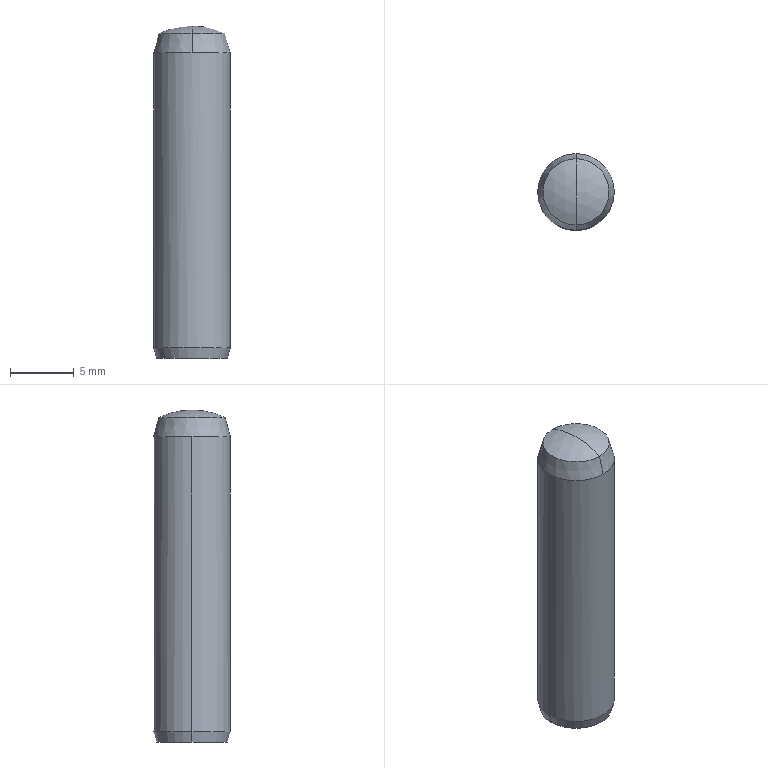Part | SolidWorks | features Chamfer 2, Cut 2, Extrusion 1, RevCut 1, Revolution 1 | 1 solid | 17 faces | box 6 x 6 x 26 mm | volume 614.212 mm3 | cone 8 | cylinder 6 | sphere 2 | plane 1 | commonest cylinder face diameters 3.464 x2 4.3 x2 6 x2
STEP:
#1=CARTESIAN_POINT('',(1.732,0.,1.418));
#2=VERTEX_POINT('',#1);
#3=CARTESIAN_POINT('',(-1.732,0.,1.418));
#4=VERTEX_POINT('',#3);
#5=CARTESIAN_POINT('',(0.,0.,1.418));
#6=DIRECTION('',(0.,0.,-1.));
#7=DIRECTION('',(-1.,0.,0.));
#8=AXIS2_PLACEMENT_3D('',#5,#6,#7);
#9=CIRCLE('',#8,1.732);
#10=EDGE_CURVE('',#2,#4,#9,.T.);
#11=ORIENTED_EDGE('',*,*,#10,.F.);
#12=CARTESIAN_POINT('',(2.15,0.,1.));
#13=VERTEX_POINT('',#12);
#14=CARTESIAN_POINT('',(2.15,0.,1.));
#15=DIRECTION('',(0.7071,0.,-0.7071));
#16=VECTOR('',#15,1000.);
#17=LINE('',#14,#16);
#18=EDGE_CURVE('',#2,#13,#17,.T.);
#19=ORIENTED_EDGE('',*,*,#18,.T.);
#20=CARTESIAN_POINT('',(-2.15,0.,1.));
#21=VERTEX_POINT('',#20);
#22=CARTESIAN_POINT('',(0.,0.,1.));
#23=DIRECTION('',(0.,0.,-1.));
#24=DIRECTION('',(-1.,0.,0.));
#25=AXIS2_PLACEMENT_3D('',#22,#23,#24);
#26=CIRCLE('',#25,2.15);
#27=EDGE_CURVE('',#13,#21,#26,.T.);
#28=ORIENTED_EDGE('',*,*,#27,.T.);
#29=CARTESIAN_POINT('',(-2.15,0.,1.));
#30=DIRECTION('',(-0.7071,0.,-0.7071));
#31=VECTOR('',#30,1000.);
#32=LINE('',#29,#31);
#33=EDGE_CURVE('',#4,#21,#32,.T.);
#34=ORIENTED_EDGE('',*,*,#33,.F.);
#35=EDGE_LOOP('',(#11,#19,#28,#34));
#36=FACE_OUTER_BOUND('',#35,.T.);
#37=CARTESIAN_POINT('',(0.,0.,1.));
#38=DIRECTION('',(0.,0.,-1.));
#39=DIRECTION('',(-1.,0.,0.));
#40=AXIS2_PLACEMENT_3D('',#37,#38,#39);
#41=CONICAL_SURFACE('',#40,2.15,0.7854);
#42=ADVANCED_FACE('',(#36),#41,.F.);
#43=CARTESIAN_POINT('',(-1.732,0.,10.));
#44=VERTEX_POINT('',#43);
#45=CARTESIAN_POINT('',(1.732,0.,10.));
#46=VERTEX_POINT('',#45);
#47=CARTESIAN_POINT('',(0.,0.,10.));
#48=DIRECTION('',(0.,0.,1.));
#49=DIRECTION('',(1.,0.,0.));
#50=AXIS2_PLACEMENT_3D('',#47,#48,#49);
#51=CIRCLE('',#50,1.732);
#52=EDGE_CURVE('',#44,#46,#51,.T.);
#53=ORIENTED_EDGE('',*,*,#52,.T.);
#54=CARTESIAN_POINT('',(1.732,0.,10.));
#55=DIRECTION('',(0.,0.,-1.));
#56=VECTOR('',#55,1000.);
#57=LINE('',#54,#56);
#58=EDGE_CURVE('',#46,#2,#57,.T.);
#59=ORIENTED_EDGE('',*,*,#58,.T.);
#60=ORIENTED_EDGE('',*,*,#10,.T.);
#61=CARTESIAN_POINT('',(-1.732,0.,10.));
#62=DIRECTION('',(0.,0.,-1.));
#63=VECTOR('',#62,1000.);
#64=LINE('',#61,#63);
#65=EDGE_CURVE('',#44,#4,#64,.T.);
#66=ORIENTED_EDGE('',*,*,#65,.F.);
#67=EDGE_LOOP('',(#53,#59,#60,#66));
#68=FACE_OUTER_BOUND('',#67,.T.);
#69=CARTESIAN_POINT('',(0.,0.,10.));
#70=DIRECTION('',(0.,0.,-1.));
#71=DIRECTION('',(-1.,0.,0.));
#72=AXIS2_PLACEMENT_3D('',#69,#70,#71);
#73=CYLINDRICAL_SURFACE('',#72,1.732);
#74=ADVANCED_FACE('',(#68),#73,.F.);
#75=CARTESIAN_POINT('',(0.,0.,11.));
#76=VERTEX_POINT('',#75);
#77=CARTESIAN_POINT('',(-1.732,0.,10.));
#78=DIRECTION('',(-0.866,0.,-0.5));
#79=VECTOR('',#78,1000.);
#80=LINE('',#77,#79);
#81=EDGE_CURVE('',#76,#44,#80,.T.);
#82=ORIENTED_EDGE('',*,*,#81,.F.);
#83=CARTESIAN_POINT('',(1.732,0.,10.));
#84=DIRECTION('',(0.866,0.,-0.5));
#85=VECTOR('',#84,1000.);
#86=LINE('',#83,#85);
#87=EDGE_CURVE('',#76,#46,#86,.T.);
#88=ORIENTED_EDGE('',*,*,#87,.T.);
#89=ORIENTED_EDGE('',*,*,#52,.F.);
#90=EDGE_LOOP('',(#82,#88,#89));
#91=FACE_OUTER_BOUND('',#90,.T.);
#92=CARTESIAN_POINT('',(0.,0.,10.));
#93=DIRECTION('',(0.,0.,-1.));
#94=DIRECTION('',(-1.,0.,0.));
#95=AXIS2_PLACEMENT_3D('',#92,#93,#94);
#96=CONICAL_SURFACE('',#95,1.732,1.047);
#97=ADVANCED_FACE('',(#91),#96,.F.);
#98=ORIENTED_EDGE('',*,*,#27,.F.);
#99=CARTESIAN_POINT('',(2.15,0.,0.));
#100=VERTEX_POINT('',#99);
#101=CARTESIAN_POINT('',(2.15,0.,1.));
#102=DIRECTION('',(0.,0.,-1.));
#103=VECTOR('',#102,1000.);
#104=LINE('',#101,#103);
#105=EDGE_CURVE('',#13,#100,#104,.T.);
#106=ORIENTED_EDGE('',*,*,#105,.T.);
#107=CARTESIAN_POINT('',(-2.15,0.,0.));
#108=VERTEX_POINT('',#107);
#109=CARTESIAN_POINT('',(0.,0.,0.));
#110=DIRECTION('',(0.,0.,-1.));
#111=DIRECTION('',(-1.,0.,0.));
#112=AXIS2_PLACEMENT_3D('',#109,#110,#111);
#113=CIRCLE('',#112,2.15);
#114=EDGE_CURVE('',#100,#108,#113,.T.);
#115=ORIENTED_EDGE('',*,*,#114,.T.);
#116=CARTESIAN_POINT('',(-2.15,0.,1.));
#117=DIRECTION('',(0.,0.,-1.));
#118=VECTOR('',#117,1000.);
#119=LINE('',#116,#118);
#120=EDGE_CURVE('',#21,#108,#119,.T.);
#121=ORIENTED_EDGE('',*,*,#120,.F.);
#122=EDGE_LOOP('',(#98,#106,#115,#121));
#123=FACE_OUTER_BOUND('',#122,.T.);
#124=CARTESIAN_POINT('',(0.,0.,1.));
#125=DIRECTION('',(0.,0.,-1.));
#126=DIRECTION('',(-1.,0.,0.));
#127=AXIS2_PLACEMENT_3D('',#124,#125,#126);
#128=CYLINDRICAL_SURFACE('',#127,2.15);
#129=ADVANCED_FACE('',(#123),#128,.F.);
#130=CARTESIAN_POINT('',(-2.786,0.,0.));
#131=VERTEX_POINT('',#130);
#132=CARTESIAN_POINT('',(2.786,0.,0.));
#133=VERTEX_POINT('',#132);
#134=CARTESIAN_POINT('',(0.,0.,0.));
#135=DIRECTION('',(0.,0.,-1.));
#136=DIRECTION('',(1.,0.,0.));
#137=AXIS2_PLACEMENT_3D('',#134,#135,#136);
#138=CIRCLE('',#137,2.786);
#139=EDGE_CURVE('',#131,#133,#138,.T.);
#140=ORIENTED_EDGE('',*,*,#139,.F.);
#141=CARTESIAN_POINT('',(-3.,0.,0.8));
#142=VERTEX_POINT('',#141);
#143=CARTESIAN_POINT('',(-3.,0.,0.8));
#144=DIRECTION('',(-0.2588,0.,0.9659));
#145=VECTOR('',#144,1000.);
#146=LINE('',#143,#145);
#147=EDGE_CURVE('',#131,#142,#146,.T.);
#148=ORIENTED_EDGE('',*,*,#147,.T.);
#149=CARTESIAN_POINT('',(3.,0.,0.8));
#150=VERTEX_POINT('',#149);
#151=CARTESIAN_POINT('',(0.,0.,0.8));
#152=DIRECTION('',(0.,0.,1.));
#153=DIRECTION('',(1.,0.,0.));
#154=AXIS2_PLACEMENT_3D('',#151,#152,#153);
#155=CIRCLE('',#154,3.);
#156=EDGE_CURVE('',#150,#142,#155,.T.);
#157=ORIENTED_EDGE('',*,*,#156,.F.);
#158=CARTESIAN_POINT('',(3.,0.,0.8));
#159=DIRECTION('',(0.2588,0.,0.9659));
#160=VECTOR('',#159,1000.);
#161=LINE('',#158,#160);
#162=EDGE_CURVE('',#133,#150,#161,.T.);
#163=ORIENTED_EDGE('',*,*,#162,.F.);
#164=EDGE_LOOP('',(#140,#148,#157,#163));
#165=FACE_OUTER_BOUND('',#164,.T.);
#166=CARTESIAN_POINT('',(0.,0.,0.8));
#167=DIRECTION('',(0.,0.,1.));
#168=DIRECTION('',(1.,0.,0.));
#169=AXIS2_PLACEMENT_3D('',#166,#167,#168);
#170=CONICAL_SURFACE('',#169,3.,0.2618);
#171=ADVANCED_FACE('',(#165),#170,.T.);
#172=CARTESIAN_POINT('',(0.,0.,26.));
#173=VERTEX_POINT('',#172);
#174=CARTESIAN_POINT('',(0.,2.596,25.41));
#175=VERTEX_POINT('',#174);
#176=CARTESIAN_POINT('',(0.,0.,20.));
#177=DIRECTION('',(-1.,0.,0.));
#178=DIRECTION('',(0.,0.,1.));
#179=AXIS2_PLACEMENT_3D('',#176,#177,#178);
#180=CIRCLE('',#179,6.);
#181=EDGE_CURVE('',#173,#175,#180,.T.);
#182=ORIENTED_EDGE('',*,*,#181,.F.);
#183=CARTESIAN_POINT('',(0.,-2.596,25.41));
#184=VERTEX_POINT('',#183);
#185=CARTESIAN_POINT('',(0.,0.,20.));
#186=DIRECTION('',(1.,0.,0.));
#187=DIRECTION('',(0.,1.,0.));
#188=AXIS2_PLACEMENT_3D('',#185,#186,#187);
#189=CIRCLE('',#188,6.);
#190=EDGE_CURVE('',#173,#184,#189,.T.);
#191=ORIENTED_EDGE('',*,*,#190,.T.);
#192=CARTESIAN_POINT('',(0.,0.,25.41));
#193=DIRECTION('',(0.,0.,-1.));
#194=DIRECTION('',(0.,1.,0.));
#195=AXIS2_PLACEMENT_3D('',#192,#193,#194);
#196=CIRCLE('',#195,2.596);
#197=EDGE_CURVE('',#175,#184,#196,.T.);
#198=ORIENTED_EDGE('',*,*,#197,.F.);
#199=EDGE_LOOP('',(#182,#191,#198));
#200=FACE_OUTER_BOUND('',#199,.T.);
#201=CARTESIAN_POINT('',(0.,0.,20.));
#202=DIRECTION('',(1.,0.,0.));
#203=DIRECTION('',(0.,1.,0.));
#204=AXIS2_PLACEMENT_3D('',#201,#202,#203);
#205=SPHERICAL_SURFACE('',#204,6.);
#206=ADVANCED_FACE('',(#200),#205,.T.);
#207=ORIENTED_EDGE('',*,*,#197,.T.);
#208=CARTESIAN_POINT('',(0.,-3.,23.9));
#209=VERTEX_POINT('',#208);
#210=CARTESIAN_POINT('',(0.,-3.,23.9));
#211=DIRECTION('',(0.,-0.2588,-0.9659));
#212=VECTOR('',#211,1000.);
#213=LINE('',#210,#212);
#214=EDGE_CURVE('',#184,#209,#213,.T.);
#215=ORIENTED_EDGE('',*,*,#214,.T.);
#216=CARTESIAN_POINT('',(3.,0.,23.9));
#217=VERTEX_POINT('',#216);
#218=CARTESIAN_POINT('',(0.,0.,23.9));
#219=DIRECTION('',(0.,0.,1.));
#220=DIRECTION('',(1.,0.,0.));
#221=AXIS2_PLACEMENT_3D('',#218,#219,#220);
#222=CIRCLE('',#221,3.);
#223=EDGE_CURVE('',#209,#217,#222,.T.);
#224=ORIENTED_EDGE('',*,*,#223,.T.);
#225=CARTESIAN_POINT('',(0.,3.,23.9));
#226=VERTEX_POINT('',#225);
#227=CARTESIAN_POINT('',(0.,0.,23.9));
#228=DIRECTION('',(0.,0.,1.));
#229=DIRECTION('',(1.,0.,0.));
#230=AXIS2_PLACEMENT_3D('',#227,#228,#229);
#231=CIRCLE('',#230,3.);
#232=EDGE_CURVE('',#217,#226,#231,.T.);
#233=ORIENTED_EDGE('',*,*,#232,.T.);
#234=CARTESIAN_POINT('',(0.,3.,23.9));
#235=DIRECTION('',(0.,0.2588,-0.9659));
#236=VECTOR('',#235,1000.);
#237=LINE('',#234,#236);
#238=EDGE_CURVE('',#175,#226,#237,.T.);
#239=ORIENTED_EDGE('',*,*,#238,.F.);
#240=EDGE_LOOP('',(#207,#215,#224,#233,#239));
#241=FACE_OUTER_BOUND('',#240,.T.);
#242=CARTESIAN_POINT('',(0.,0.,23.9));
#243=DIRECTION('',(0.,0.,-1.));
#244=DIRECTION('',(0.,1.,0.));
#245=AXIS2_PLACEMENT_3D('',#242,#243,#244);
#246=CONICAL_SURFACE('',#245,3.,0.2618);
#247=ADVANCED_FACE('',(#241),#246,.T.);
#248=ORIENTED_EDGE('',*,*,#232,.F.);
#249=CARTESIAN_POINT('',(3.,0.,23.9));
#250=DIRECTION('',(0.,0.,-1.));
#251=VECTOR('',#250,1000.);
#252=LINE('',#249,#251);
#253=EDGE_CURVE('',#217,#150,#252,.T.);
#254=ORIENTED_EDGE('',*,*,#253,.T.);
#255=ORIENTED_EDGE('',*,*,#156,.T.);
#256=CARTESIAN_POINT('',(-3.,0.,23.9));
#257=VERTEX_POINT('',#256);
#258=CARTESIAN_POINT('',(-3.,0.,23.9));
#259=DIRECTION('',(0.,0.,-1.));
#260=VECTOR('',#259,1000.);
#261=LINE('',#258,#260);
#262=EDGE_CURVE('',#257,#142,#261,.T.);
#263=ORIENTED_EDGE('',*,*,#262,.F.);
#264=CARTESIAN_POINT('',(0.,0.,23.9));
#265=DIRECTION('',(0.,0.,1.));
#266=DIRECTION('',(1.,0.,0.));
#267=AXIS2_PLACEMENT_3D('',#264,#265,#266);
#268=CIRCLE('',#267,3.);
#269=EDGE_CURVE('',#226,#257,#268,.T.);
#270=ORIENTED_EDGE('',*,*,#269,.F.);
#271=EDGE_LOOP('',(#248,#254,#255,#263,#270));
#272=FACE_OUTER_BOUND('',#271,.T.);
#273=CARTESIAN_POINT('',(0.,0.,23.9));
#274=DIRECTION('',(0.,0.,-1.));
#275=DIRECTION('',(-1.,0.,0.));
#276=AXIS2_PLACEMENT_3D('',#273,#274,#275);
#277=CYLINDRICAL_SURFACE('',#276,3.);
#278=ADVANCED_FACE('',(#272),#277,.T.);
#279=ORIENTED_EDGE('',*,*,#253,.F.);
#280=ORIENTED_EDGE('',*,*,#223,.F.);
#281=CARTESIAN_POINT('',(0.,0.,23.9));
#282=DIRECTION('',(0.,0.,1.));
#283=DIRECTION('',(1.,0.,0.));
#284=AXIS2_PLACEMENT_3D('',#281,#282,#283);
#285=CIRCLE('',#284,3.);
#286=EDGE_CURVE('',#257,#209,#285,.T.);
#287=ORIENTED_EDGE('',*,*,#286,.F.);
#288=ORIENTED_EDGE('',*,*,#262,.T.);
#289=CARTESIAN_POINT('',(0.,0.,0.8));
#290=DIRECTION('',(0.,0.,1.));
#291=DIRECTION('',(1.,0.,0.));
#292=AXIS2_PLACEMENT_3D('',#289,#290,#291);
#293=CIRCLE('',#292,3.);
#294=EDGE_CURVE('',#142,#150,#293,.T.);
#295=ORIENTED_EDGE('',*,*,#294,.T.);
#296=EDGE_LOOP('',(#279,#280,#287,#288,#295));
#297=FACE_OUTER_BOUND('',#296,.T.);
#298=CARTESIAN_POINT('',(0.,0.,23.9));
#299=DIRECTION('',(0.,0.,-1.));
#300=DIRECTION('',(-1.,0.,0.));
#301=AXIS2_PLACEMENT_3D('',#298,#299,#300);
#302=CYLINDRICAL_SURFACE('',#301,3.);
#303=ADVANCED_FACE('',(#297),#302,.T.);
#304=CARTESIAN_POINT('',(0.,0.,0.));
#305=DIRECTION('',(0.,0.,-1.));
#306=DIRECTION('',(-1.,0.,0.));
#307=AXIS2_PLACEMENT_3D('',#304,#305,#306);
#308=CIRCLE('',#307,2.15);
#309=EDGE_CURVE('',#108,#100,#308,.T.);
#310=ORIENTED_EDGE('',*,*,#309,.F.);
#311=ORIENTED_EDGE('',*,*,#114,.F.);
#312=EDGE_LOOP('',(#310,#311));
#313=FACE_BOUND('',#312,.T.);
#314=CARTESIAN_POINT('',(0.,0.,0.));
#315=DIRECTION('',(0.,0.,-1.));
#316=DIRECTION('',(1.,0.,0.));
#317=AXIS2_PLACEMENT_3D('',#314,#315,#316);
#318=CIRCLE('',#317,2.786);
#319=EDGE_CURVE('',#133,#131,#318,.T.);
#320=ORIENTED_EDGE('',*,*,#319,.T.);
#321=ORIENTED_EDGE('',*,*,#139,.T.);
#322=EDGE_LOOP('',(#320,#321));
#323=FACE_OUTER_BOUND('',#322,.T.);
#324=CARTESIAN_POINT('',(0.,0.,0.));
#325=DIRECTION('',(0.,0.,1.));
#326=DIRECTION('',(1.,0.,0.));
#327=AXIS2_PLACEMENT_3D('',#324,#325,#326);
#328=PLANE('',#327);
#329=ADVANCED_FACE('',(#313,#323),#328,.F.);
#330=ORIENTED_EDGE('',*,*,#214,.F.);
#331=CARTESIAN_POINT('',(0.,0.,25.41));
#332=DIRECTION('',(0.,0.,-1.));
#333=DIRECTION('',(0.,1.,0.));
#334=AXIS2_PLACEMENT_3D('',#331,#332,#333);
#335=CIRCLE('',#334,2.596);
#336=EDGE_CURVE('',#184,#175,#335,.T.);
#337=ORIENTED_EDGE('',*,*,#336,.T.);
#338=ORIENTED_EDGE('',*,*,#238,.T.);
#339=ORIENTED_EDGE('',*,*,#269,.T.);
#340=ORIENTED_EDGE('',*,*,#286,.T.);
#341=EDGE_LOOP('',(#330,#337,#338,#339,#340));
#342=FACE_OUTER_BOUND('',#341,.T.);
#343=CARTESIAN_POINT('',(0.,0.,23.9));
#344=DIRECTION('',(0.,0.,-1.));
#345=DIRECTION('',(0.,1.,0.));
#346=AXIS2_PLACEMENT_3D('',#343,#344,#345);
#347=CONICAL_SURFACE('',#346,3.,0.2618);
#348=ADVANCED_FACE('',(#342),#347,.T.);
#349=ORIENTED_EDGE('',*,*,#190,.F.);
#350=ORIENTED_EDGE('',*,*,#181,.T.);
#351=ORIENTED_EDGE('',*,*,#336,.F.);
#352=EDGE_LOOP('',(#349,#350,#351));
#353=FACE_OUTER_BOUND('',#352,.T.);
#354=CARTESIAN_POINT('',(0.,0.,20.));
#355=DIRECTION('',(1.,0.,0.));
#356=DIRECTION('',(0.,1.,0.));
#357=AXIS2_PLACEMENT_3D('',#354,#355,#356);
#358=SPHERICAL_SURFACE('',#357,6.);
#359=ADVANCED_FACE('',(#353),#358,.T.);
#360=ORIENTED_EDGE('',*,*,#147,.F.);
#361=ORIENTED_EDGE('',*,*,#319,.F.);
#362=ORIENTED_EDGE('',*,*,#162,.T.);
#363=ORIENTED_EDGE('',*,*,#294,.F.);
#364=EDGE_LOOP('',(#360,#361,#362,#363));
#365=FACE_OUTER_BOUND('',#364,.T.);
#366=CARTESIAN_POINT('',(0.,0.,0.8));
#367=DIRECTION('',(0.,0.,1.));
#368=DIRECTION('',(1.,0.,0.));
#369=AXIS2_PLACEMENT_3D('',#366,#367,#368);
#370=CONICAL_SURFACE('',#369,3.,0.2618);
#371=ADVANCED_FACE('',(#365),#370,.T.);
#372=ORIENTED_EDGE('',*,*,#105,.F.);
#373=CARTESIAN_POINT('',(0.,0.,1.));
#374=DIRECTION('',(0.,0.,-1.));
#375=DIRECTION('',(-1.,0.,0.));
#376=AXIS2_PLACEMENT_3D('',#373,#374,#375);
#377=CIRCLE('',#376,2.15);
#378=EDGE_CURVE('',#21,#13,#377,.T.);
#379=ORIENTED_EDGE('',*,*,#378,.F.);
#380=ORIENTED_EDGE('',*,*,#120,.T.);
#381=ORIENTED_EDGE('',*,*,#309,.T.);
#382=EDGE_LOOP('',(#372,#379,#380,#381));
#383=FACE_OUTER_BOUND('',#382,.T.);
#384=CARTESIAN_POINT('',(0.,0.,1.));
#385=DIRECTION('',(0.,0.,-1.));
#386=DIRECTION('',(-1.,0.,0.));
#387=AXIS2_PLACEMENT_3D('',#384,#385,#386);
#388=CYLINDRICAL_SURFACE('',#387,2.15);
#389=ADVANCED_FACE('',(#383),#388,.F.);
#390=ORIENTED_EDGE('',*,*,#87,.F.);
#391=ORIENTED_EDGE('',*,*,#81,.T.);
#392=CARTESIAN_POINT('',(0.,0.,10.));
#393=DIRECTION('',(0.,0.,1.));
#394=DIRECTION('',(1.,0.,0.));
#395=AXIS2_PLACEMENT_3D('',#392,#393,#394);
#396=CIRCLE('',#395,1.732);
#397=EDGE_CURVE('',#46,#44,#396,.T.);
#398=ORIENTED_EDGE('',*,*,#397,.F.);
#399=EDGE_LOOP('',(#390,#391,#398));
#400=FACE_OUTER_BOUND('',#399,.T.);
#401=CARTESIAN_POINT('',(0.,0.,10.));
#402=DIRECTION('',(0.,0.,-1.));
#403=DIRECTION('',(-1.,0.,0.));
#404=AXIS2_PLACEMENT_3D('',#401,#402,#403);
#405=CONICAL_SURFACE('',#404,1.732,1.047);
#406=ADVANCED_FACE('',(#400),#405,.F.);
#407=ORIENTED_EDGE('',*,*,#58,.F.);
#408=ORIENTED_EDGE('',*,*,#397,.T.);
#409=ORIENTED_EDGE('',*,*,#65,.T.);
#410=CARTESIAN_POINT('',(0.,0.,1.418));
#411=DIRECTION('',(0.,0.,-1.));
#412=DIRECTION('',(-1.,0.,0.));
#413=AXIS2_PLACEMENT_3D('',#410,#411,#412);
#414=CIRCLE('',#413,1.732);
#415=EDGE_CURVE('',#4,#2,#414,.T.);
#416=ORIENTED_EDGE('',*,*,#415,.T.);
#417=EDGE_LOOP('',(#407,#408,#409,#416));
#418=FACE_OUTER_BOUND('',#417,.T.);
#419=CARTESIAN_POINT('',(0.,0.,10.));
#420=DIRECTION('',(0.,0.,-1.));
#421=DIRECTION('',(-1.,0.,0.));
#422=AXIS2_PLACEMENT_3D('',#419,#420,#421);
#423=CYLINDRICAL_SURFACE('',#422,1.732);
#424=ADVANCED_FACE('',(#418),#423,.F.);
#425=ORIENTED_EDGE('',*,*,#18,.F.);
#426=ORIENTED_EDGE('',*,*,#415,.F.);
#427=ORIENTED_EDGE('',*,*,#33,.T.);
#428=ORIENTED_EDGE('',*,*,#378,.T.);
#429=EDGE_LOOP('',(#425,#426,#427,#428));
#430=FACE_OUTER_BOUND('',#429,.T.);
#431=CARTESIAN_POINT('',(0.,0.,1.));
#432=DIRECTION('',(0.,0.,-1.));
#433=DIRECTION('',(-1.,0.,0.));
#434=AXIS2_PLACEMENT_3D('',#431,#432,#433);
#435=CONICAL_SURFACE('',#434,2.15,0.7854);
#436=ADVANCED_FACE('',(#430),#435,.F.);
#437=CLOSED_SHELL('',(#42,#74,#97,#129,#171,#206,#247,#278,#303,#329,#348,#359,#371,#389,#406,#424,#436));
#438=MANIFOLD_SOLID_BREP('',#437);
#439=CARTESIAN_POINT('',(0.,0.,0.));
#440=DIRECTION('',(0.,0.,1.));
#441=DIRECTION('',(1.,0.,0.));
#442=AXIS2_PLACEMENT_3D('',#439,#440,#441);
#443=(LENGTH_UNIT()NAMED_UNIT(*)SI_UNIT(.MILLI.,.METRE.));
#444=UNCERTAINTY_MEASURE_WITH_UNIT(LENGTH_MEASURE(0.00001),#443,'','');
#445=(NAMED_UNIT(*)PLANE_ANGLE_UNIT()SI_UNIT($,.RADIAN.));
#446=(NAMED_UNIT(*)SI_UNIT($,.STERADIAN.)SOLID_ANGLE_UNIT());
#447=(GEOMETRIC_REPRESENTATION_CONTEXT(3)GLOBAL_UNCERTAINTY_ASSIGNED_CONTEXT((#444))GLOBAL_UNIT_ASSIGNED_CONTEXT((#443,#445,#446))REPRESENTATION_CONTEXT('',''));
#448=ADVANCED_BREP_SHAPE_REPRESENTATION('',(#438,#442),#447);